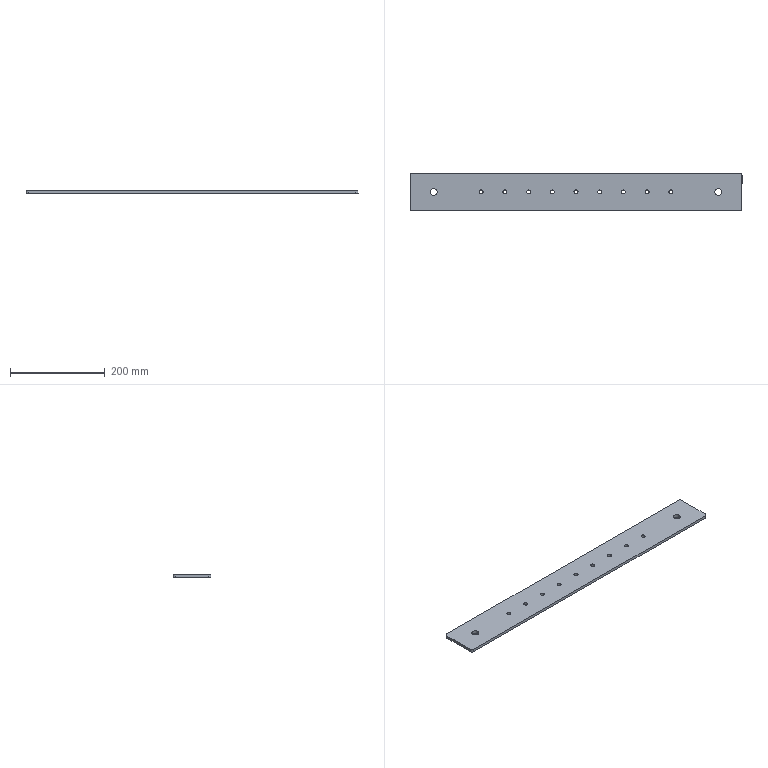Part | STEP file | 750038460 | 1 solid | 32 faces | box 700 x 80 x 6 mm | volume 330686 mm3 | cylinder 26 | plane 6 | commonest cylinder face diameters 8.5 x18 10 x4 15 x4
STEP:
#1=CARTESIAN_POINT('',(-607.5,0.,0.));
#2=VERTEX_POINT('',#1);
#3=CARTESIAN_POINT('',(-592.5,0.,0.));
#4=VERTEX_POINT('',#3);
#5=CARTESIAN_POINT('',(-600.,0.,0.));
#6=DIRECTION('',(0.,0.,1.));
#7=DIRECTION('',(1.,0.,0.));
#8=AXIS2_PLACEMENT_3D('',#5,#6,#7);
#9=CIRCLE('',#8,7.5);
#10=EDGE_CURVE('',#2,#4,#9,.T.);
#11=ORIENTED_EDGE('',*,*,#10,.F.);
#12=CARTESIAN_POINT('',(-607.5,0.,6.));
#13=VERTEX_POINT('',#12);
#14=CARTESIAN_POINT('',(-607.5,0.,-54994.));
#15=DIRECTION('',(0.,0.,1.));
#16=VECTOR('',#15,1000.);
#17=LINE('',#14,#16);
#18=EDGE_CURVE('',#2,#13,#17,.T.);
#19=ORIENTED_EDGE('',*,*,#18,.T.);
#20=CARTESIAN_POINT('',(-592.5,0.,6.));
#21=VERTEX_POINT('',#20);
#22=CARTESIAN_POINT('',(-600.,0.,6.));
#23=DIRECTION('',(0.,0.,-1.));
#24=DIRECTION('',(1.,0.,0.));
#25=AXIS2_PLACEMENT_3D('',#22,#23,#24);
#26=CIRCLE('',#25,7.5);
#27=EDGE_CURVE('',#21,#13,#26,.T.);
#28=ORIENTED_EDGE('',*,*,#27,.F.);
#29=CARTESIAN_POINT('',(-592.5,0.,-54994.));
#30=DIRECTION('',(0.,0.,1.));
#31=VECTOR('',#30,1000.);
#32=LINE('',#29,#31);
#33=EDGE_CURVE('',#4,#21,#32,.T.);
#34=ORIENTED_EDGE('',*,*,#33,.F.);
#35=EDGE_LOOP('',(#11,#19,#28,#34));
#36=FACE_OUTER_BOUND('',#35,.T.);
#37=CARTESIAN_POINT('',(-600.,0.,-54994.));
#38=DIRECTION('',(0.,0.,1.));
#39=DIRECTION('',(1.,0.,0.));
#40=AXIS2_PLACEMENT_3D('',#37,#38,#39);
#41=CYLINDRICAL_SURFACE('',#40,7.5);
#42=ADVANCED_FACE('',(#36),#41,.F.);
#43=CARTESIAN_POINT('',(-504.25,0.,0.));
#44=VERTEX_POINT('',#43);
#45=CARTESIAN_POINT('',(-495.75,0.,0.));
#46=VERTEX_POINT('',#45);
#47=CARTESIAN_POINT('',(-500.,0.,0.));
#48=DIRECTION('',(0.,0.,1.));
#49=DIRECTION('',(1.,0.,0.));
#50=AXIS2_PLACEMENT_3D('',#47,#48,#49);
#51=CIRCLE('',#50,4.25);
#52=EDGE_CURVE('',#44,#46,#51,.T.);
#53=ORIENTED_EDGE('',*,*,#52,.F.);
#54=CARTESIAN_POINT('',(-504.25,0.,6.));
#55=VERTEX_POINT('',#54);
#56=CARTESIAN_POINT('',(-504.25,0.,-54994.));
#57=DIRECTION('',(0.,0.,1.));
#58=VECTOR('',#57,1000.);
#59=LINE('',#56,#58);
#60=EDGE_CURVE('',#44,#55,#59,.T.);
#61=ORIENTED_EDGE('',*,*,#60,.T.);
#62=CARTESIAN_POINT('',(-495.75,0.,6.));
#63=VERTEX_POINT('',#62);
#64=CARTESIAN_POINT('',(-500.,0.,6.));
#65=DIRECTION('',(0.,0.,-1.));
#66=DIRECTION('',(1.,0.,0.));
#67=AXIS2_PLACEMENT_3D('',#64,#65,#66);
#68=CIRCLE('',#67,4.25);
#69=EDGE_CURVE('',#63,#55,#68,.T.);
#70=ORIENTED_EDGE('',*,*,#69,.F.);
#71=CARTESIAN_POINT('',(-495.75,0.,-54994.));
#72=DIRECTION('',(0.,0.,1.));
#73=VECTOR('',#72,1000.);
#74=LINE('',#71,#73);
#75=EDGE_CURVE('',#46,#63,#74,.T.);
#76=ORIENTED_EDGE('',*,*,#75,.F.);
#77=EDGE_LOOP('',(#53,#61,#70,#76));
#78=FACE_OUTER_BOUND('',#77,.T.);
#79=CARTESIAN_POINT('',(-500.,0.,-54994.));
#80=DIRECTION('',(0.,0.,1.));
#81=DIRECTION('',(1.,0.,0.));
#82=AXIS2_PLACEMENT_3D('',#79,#80,#81);
#83=CYLINDRICAL_SURFACE('',#82,4.25);
#84=ADVANCED_FACE('',(#78),#83,.F.);
#85=CARTESIAN_POINT('',(-454.25,0.,0.));
#86=VERTEX_POINT('',#85);
#87=CARTESIAN_POINT('',(-445.75,0.,0.));
#88=VERTEX_POINT('',#87);
#89=CARTESIAN_POINT('',(-450.,0.,0.));
#90=DIRECTION('',(0.,0.,1.));
#91=DIRECTION('',(1.,0.,0.));
#92=AXIS2_PLACEMENT_3D('',#89,#90,#91);
#93=CIRCLE('',#92,4.25);
#94=EDGE_CURVE('',#86,#88,#93,.T.);
#95=ORIENTED_EDGE('',*,*,#94,.F.);
#96=CARTESIAN_POINT('',(-454.25,0.,6.));
#97=VERTEX_POINT('',#96);
#98=CARTESIAN_POINT('',(-454.25,0.,-54994.));
#99=DIRECTION('',(0.,0.,1.));
#100=VECTOR('',#99,1000.);
#101=LINE('',#98,#100);
#102=EDGE_CURVE('',#86,#97,#101,.T.);
#103=ORIENTED_EDGE('',*,*,#102,.T.);
#104=CARTESIAN_POINT('',(-445.75,0.,6.));
#105=VERTEX_POINT('',#104);
#106=CARTESIAN_POINT('',(-450.,0.,6.));
#107=DIRECTION('',(0.,0.,-1.));
#108=DIRECTION('',(1.,0.,0.));
#109=AXIS2_PLACEMENT_3D('',#106,#107,#108);
#110=CIRCLE('',#109,4.25);
#111=EDGE_CURVE('',#105,#97,#110,.T.);
#112=ORIENTED_EDGE('',*,*,#111,.F.);
#113=CARTESIAN_POINT('',(-445.75,0.,-54994.));
#114=DIRECTION('',(0.,0.,1.));
#115=VECTOR('',#114,1000.);
#116=LINE('',#113,#115);
#117=EDGE_CURVE('',#88,#105,#116,.T.);
#118=ORIENTED_EDGE('',*,*,#117,.F.);
#119=EDGE_LOOP('',(#95,#103,#112,#118));
#120=FACE_OUTER_BOUND('',#119,.T.);
#121=CARTESIAN_POINT('',(-450.,0.,-54994.));
#122=DIRECTION('',(0.,0.,1.));
#123=DIRECTION('',(1.,0.,0.));
#124=AXIS2_PLACEMENT_3D('',#121,#122,#123);
#125=CYLINDRICAL_SURFACE('',#124,4.25);
#126=ADVANCED_FACE('',(#120),#125,.F.);
#127=CARTESIAN_POINT('',(-404.25,0.,0.));
#128=VERTEX_POINT('',#127);
#129=CARTESIAN_POINT('',(-395.75,0.,0.));
#130=VERTEX_POINT('',#129);
#131=CARTESIAN_POINT('',(-400.,0.,0.));
#132=DIRECTION('',(0.,0.,1.));
#133=DIRECTION('',(1.,0.,0.));
#134=AXIS2_PLACEMENT_3D('',#131,#132,#133);
#135=CIRCLE('',#134,4.25);
#136=EDGE_CURVE('',#128,#130,#135,.T.);
#137=ORIENTED_EDGE('',*,*,#136,.F.);
#138=CARTESIAN_POINT('',(-404.25,0.,6.));
#139=VERTEX_POINT('',#138);
#140=CARTESIAN_POINT('',(-404.25,0.,-54994.));
#141=DIRECTION('',(0.,0.,1.));
#142=VECTOR('',#141,1000.);
#143=LINE('',#140,#142);
#144=EDGE_CURVE('',#128,#139,#143,.T.);
#145=ORIENTED_EDGE('',*,*,#144,.T.);
#146=CARTESIAN_POINT('',(-395.75,0.,6.));
#147=VERTEX_POINT('',#146);
#148=CARTESIAN_POINT('',(-400.,0.,6.));
#149=DIRECTION('',(0.,0.,-1.));
#150=DIRECTION('',(1.,0.,0.));
#151=AXIS2_PLACEMENT_3D('',#148,#149,#150);
#152=CIRCLE('',#151,4.25);
#153=EDGE_CURVE('',#147,#139,#152,.T.);
#154=ORIENTED_EDGE('',*,*,#153,.F.);
#155=CARTESIAN_POINT('',(-395.75,0.,-54994.));
#156=DIRECTION('',(0.,0.,1.));
#157=VECTOR('',#156,1000.);
#158=LINE('',#155,#157);
#159=EDGE_CURVE('',#130,#147,#158,.T.);
#160=ORIENTED_EDGE('',*,*,#159,.F.);
#161=EDGE_LOOP('',(#137,#145,#154,#160));
#162=FACE_OUTER_BOUND('',#161,.T.);
#163=CARTESIAN_POINT('',(-400.,0.,-54994.));
#164=DIRECTION('',(0.,0.,1.));
#165=DIRECTION('',(1.,0.,0.));
#166=AXIS2_PLACEMENT_3D('',#163,#164,#165);
#167=CYLINDRICAL_SURFACE('',#166,4.25);
#168=ADVANCED_FACE('',(#162),#167,.F.);
#169=CARTESIAN_POINT('',(-354.25,0.,0.));
#170=VERTEX_POINT('',#169);
#171=CARTESIAN_POINT('',(-345.75,0.,0.));
#172=VERTEX_POINT('',#171);
#173=CARTESIAN_POINT('',(-350.,0.,0.));
#174=DIRECTION('',(0.,0.,1.));
#175=DIRECTION('',(1.,0.,0.));
#176=AXIS2_PLACEMENT_3D('',#173,#174,#175);
#177=CIRCLE('',#176,4.25);
#178=EDGE_CURVE('',#170,#172,#177,.T.);
#179=ORIENTED_EDGE('',*,*,#178,.F.);
#180=CARTESIAN_POINT('',(-354.25,0.,6.));
#181=VERTEX_POINT('',#180);
#182=CARTESIAN_POINT('',(-354.25,0.,-54994.));
#183=DIRECTION('',(0.,0.,1.));
#184=VECTOR('',#183,1000.);
#185=LINE('',#182,#184);
#186=EDGE_CURVE('',#170,#181,#185,.T.);
#187=ORIENTED_EDGE('',*,*,#186,.T.);
#188=CARTESIAN_POINT('',(-345.75,0.,6.));
#189=VERTEX_POINT('',#188);
#190=CARTESIAN_POINT('',(-350.,0.,6.));
#191=DIRECTION('',(0.,0.,-1.));
#192=DIRECTION('',(1.,0.,0.));
#193=AXIS2_PLACEMENT_3D('',#190,#191,#192);
#194=CIRCLE('',#193,4.25);
#195=EDGE_CURVE('',#189,#181,#194,.T.);
#196=ORIENTED_EDGE('',*,*,#195,.F.);
#197=CARTESIAN_POINT('',(-345.75,0.,-54994.));
#198=DIRECTION('',(0.,0.,1.));
#199=VECTOR('',#198,1000.);
#200=LINE('',#197,#199);
#201=EDGE_CURVE('',#172,#189,#200,.T.);
#202=ORIENTED_EDGE('',*,*,#201,.F.);
#203=EDGE_LOOP('',(#179,#187,#196,#202));
#204=FACE_OUTER_BOUND('',#203,.T.);
#205=CARTESIAN_POINT('',(-350.,0.,-54994.));
#206=DIRECTION('',(0.,0.,1.));
#207=DIRECTION('',(1.,0.,0.));
#208=AXIS2_PLACEMENT_3D('',#205,#206,#207);
#209=CYLINDRICAL_SURFACE('',#208,4.25);
#210=ADVANCED_FACE('',(#204),#209,.F.);
#211=CARTESIAN_POINT('',(-304.25,0.,0.));
#212=VERTEX_POINT('',#211);
#213=CARTESIAN_POINT('',(-295.75,0.,0.));
#214=VERTEX_POINT('',#213);
#215=CARTESIAN_POINT('',(-300.,0.,0.));
#216=DIRECTION('',(0.,0.,1.));
#217=DIRECTION('',(1.,0.,0.));
#218=AXIS2_PLACEMENT_3D('',#215,#216,#217);
#219=CIRCLE('',#218,4.25);
#220=EDGE_CURVE('',#212,#214,#219,.T.);
#221=ORIENTED_EDGE('',*,*,#220,.F.);
#222=CARTESIAN_POINT('',(-304.25,0.,6.));
#223=VERTEX_POINT('',#222);
#224=CARTESIAN_POINT('',(-304.25,0.,-54994.));
#225=DIRECTION('',(0.,0.,1.));
#226=VECTOR('',#225,1000.);
#227=LINE('',#224,#226);
#228=EDGE_CURVE('',#212,#223,#227,.T.);
#229=ORIENTED_EDGE('',*,*,#228,.T.);
#230=CARTESIAN_POINT('',(-295.75,0.,6.));
#231=VERTEX_POINT('',#230);
#232=CARTESIAN_POINT('',(-300.,0.,6.));
#233=DIRECTION('',(0.,0.,-1.));
#234=DIRECTION('',(1.,0.,0.));
#235=AXIS2_PLACEMENT_3D('',#232,#233,#234);
#236=CIRCLE('',#235,4.25);
#237=EDGE_CURVE('',#231,#223,#236,.T.);
#238=ORIENTED_EDGE('',*,*,#237,.F.);
#239=CARTESIAN_POINT('',(-295.75,0.,-54994.));
#240=DIRECTION('',(0.,0.,1.));
#241=VECTOR('',#240,1000.);
#242=LINE('',#239,#241);
#243=EDGE_CURVE('',#214,#231,#242,.T.);
#244=ORIENTED_EDGE('',*,*,#243,.F.);
#245=EDGE_LOOP('',(#221,#229,#238,#244));
#246=FACE_OUTER_BOUND('',#245,.T.);
#247=CARTESIAN_POINT('',(-300.,0.,-54994.));
#248=DIRECTION('',(0.,0.,1.));
#249=DIRECTION('',(1.,0.,0.));
#250=AXIS2_PLACEMENT_3D('',#247,#248,#249);
#251=CYLINDRICAL_SURFACE('',#250,4.25);
#252=ADVANCED_FACE('',(#246),#251,.F.);
#253=CARTESIAN_POINT('',(-254.25,0.,0.));
#254=VERTEX_POINT('',#253);
#255=CARTESIAN_POINT('',(-245.75,0.,0.));
#256=VERTEX_POINT('',#255);
#257=CARTESIAN_POINT('',(-250.,0.,0.));
#258=DIRECTION('',(0.,0.,1.));
#259=DIRECTION('',(1.,0.,0.));
#260=AXIS2_PLACEMENT_3D('',#257,#258,#259);
#261=CIRCLE('',#260,4.25);
#262=EDGE_CURVE('',#254,#256,#261,.T.);
#263=ORIENTED_EDGE('',*,*,#262,.F.);
#264=CARTESIAN_POINT('',(-254.25,0.,6.));
#265=VERTEX_POINT('',#264);
#266=CARTESIAN_POINT('',(-254.25,0.,-54994.));
#267=DIRECTION('',(0.,0.,1.));
#268=VECTOR('',#267,1000.);
#269=LINE('',#266,#268);
#270=EDGE_CURVE('',#254,#265,#269,.T.);
#271=ORIENTED_EDGE('',*,*,#270,.T.);
#272=CARTESIAN_POINT('',(-245.75,0.,6.));
#273=VERTEX_POINT('',#272);
#274=CARTESIAN_POINT('',(-250.,0.,6.));
#275=DIRECTION('',(0.,0.,-1.));
#276=DIRECTION('',(1.,0.,0.));
#277=AXIS2_PLACEMENT_3D('',#274,#275,#276);
#278=CIRCLE('',#277,4.25);
#279=EDGE_CURVE('',#273,#265,#278,.T.);
#280=ORIENTED_EDGE('',*,*,#279,.F.);
#281=CARTESIAN_POINT('',(-245.75,0.,-54994.));
#282=DIRECTION('',(0.,0.,1.));
#283=VECTOR('',#282,1000.);
#284=LINE('',#281,#283);
#285=EDGE_CURVE('',#256,#273,#284,.T.);
#286=ORIENTED_EDGE('',*,*,#285,.F.);
#287=EDGE_LOOP('',(#263,#271,#280,#286));
#288=FACE_OUTER_BOUND('',#287,.T.);
#289=CARTESIAN_POINT('',(-250.,0.,-54994.));
#290=DIRECTION('',(0.,0.,1.));
#291=DIRECTION('',(1.,0.,0.));
#292=AXIS2_PLACEMENT_3D('',#289,#290,#291);
#293=CYLINDRICAL_SURFACE('',#292,4.25);
#294=ADVANCED_FACE('',(#288),#293,.F.);
#295=CARTESIAN_POINT('',(-204.25,0.,0.));
#296=VERTEX_POINT('',#295);
#297=CARTESIAN_POINT('',(-195.75,0.,0.));
#298=VERTEX_POINT('',#297);
#299=CARTESIAN_POINT('',(-200.,0.,0.));
#300=DIRECTION('',(0.,0.,1.));
#301=DIRECTION('',(1.,0.,0.));
#302=AXIS2_PLACEMENT_3D('',#299,#300,#301);
#303=CIRCLE('',#302,4.25);
#304=EDGE_CURVE('',#296,#298,#303,.T.);
#305=ORIENTED_EDGE('',*,*,#304,.F.);
#306=CARTESIAN_POINT('',(-204.25,0.,6.));
#307=VERTEX_POINT('',#306);
#308=CARTESIAN_POINT('',(-204.25,0.,-54994.));
#309=DIRECTION('',(0.,0.,1.));
#310=VECTOR('',#309,1000.);
#311=LINE('',#308,#310);
#312=EDGE_CURVE('',#296,#307,#311,.T.);
#313=ORIENTED_EDGE('',*,*,#312,.T.);
#314=CARTESIAN_POINT('',(-195.75,0.,6.));
#315=VERTEX_POINT('',#314);
#316=CARTESIAN_POINT('',(-200.,0.,6.));
#317=DIRECTION('',(0.,0.,-1.));
#318=DIRECTION('',(1.,0.,0.));
#319=AXIS2_PLACEMENT_3D('',#316,#317,#318);
#320=CIRCLE('',#319,4.25);
#321=EDGE_CURVE('',#315,#307,#320,.T.);
#322=ORIENTED_EDGE('',*,*,#321,.F.);
#323=CARTESIAN_POINT('',(-195.75,0.,-54994.));
#324=DIRECTION('',(0.,0.,1.));
#325=VECTOR('',#324,1000.);
#326=LINE('',#323,#325);
#327=EDGE_CURVE('',#298,#315,#326,.T.);
#328=ORIENTED_EDGE('',*,*,#327,.F.);
#329=EDGE_LOOP('',(#305,#313,#322,#328));
#330=FACE_OUTER_BOUND('',#329,.T.);
#331=CARTESIAN_POINT('',(-200.,0.,-54994.));
#332=DIRECTION('',(0.,0.,1.));
#333=DIRECTION('',(1.,0.,0.));
#334=AXIS2_PLACEMENT_3D('',#331,#332,#333);
#335=CYLINDRICAL_SURFACE('',#334,4.25);
#336=ADVANCED_FACE('',(#330),#335,.F.);
#337=CARTESIAN_POINT('',(-154.25,0.,0.));
#338=VERTEX_POINT('',#337);
#339=CARTESIAN_POINT('',(-145.75,0.,0.));
#340=VERTEX_POINT('',#339);
#341=CARTESIAN_POINT('',(-150.,0.,0.));
#342=DIRECTION('',(0.,0.,1.));
#343=DIRECTION('',(1.,0.,0.));
#344=AXIS2_PLACEMENT_3D('',#341,#342,#343);
#345=CIRCLE('',#344,4.25);
#346=EDGE_CURVE('',#338,#340,#345,.T.);
#347=ORIENTED_EDGE('',*,*,#346,.F.);
#348=CARTESIAN_POINT('',(-154.25,0.,6.));
#349=VERTEX_POINT('',#348);
#350=CARTESIAN_POINT('',(-154.25,0.,-54994.));
#351=DIRECTION('',(0.,0.,1.));
#352=VECTOR('',#351,1000.);
#353=LINE('',#350,#352);
#354=EDGE_CURVE('',#338,#349,#353,.T.);
#355=ORIENTED_EDGE('',*,*,#354,.T.);
#356=CARTESIAN_POINT('',(-145.75,0.,6.));
#357=VERTEX_POINT('',#356);
#358=CARTESIAN_POINT('',(-150.,0.,6.));
#359=DIRECTION('',(0.,0.,-1.));
#360=DIRECTION('',(1.,0.,0.));
#361=AXIS2_PLACEMENT_3D('',#358,#359,#360);
#362=CIRCLE('',#361,4.25);
#363=EDGE_CURVE('',#357,#349,#362,.T.);
#364=ORIENTED_EDGE('',*,*,#363,.F.);
#365=CARTESIAN_POINT('',(-145.75,0.,-54994.));
#366=DIRECTION('',(0.,0.,1.));
#367=VECTOR('',#366,1000.);
#368=LINE('',#365,#367);
#369=EDGE_CURVE('',#340,#357,#368,.T.);
#370=ORIENTED_EDGE('',*,*,#369,.F.);
#371=EDGE_LOOP('',(#347,#355,#364,#370));
#372=FACE_OUTER_BOUND('',#371,.T.);
#373=CARTESIAN_POINT('',(-150.,0.,-54994.));
#374=DIRECTION('',(0.,0.,1.));
#375=DIRECTION('',(1.,0.,0.));
#376=AXIS2_PLACEMENT_3D('',#373,#374,#375);
#377=CYLINDRICAL_SURFACE('',#376,4.25);
#378=ADVANCED_FACE('',(#372),#377,.F.);
#379=CARTESIAN_POINT('',(-104.25,0.,0.));
#380=VERTEX_POINT('',#379);
#381=CARTESIAN_POINT('',(-95.75,0.,0.));
#382=VERTEX_POINT('',#381);
#383=CARTESIAN_POINT('',(-100.,0.,0.));
#384=DIRECTION('',(0.,0.,1.));
#385=DIRECTION('',(1.,0.,0.));
#386=AXIS2_PLACEMENT_3D('',#383,#384,#385);
#387=CIRCLE('',#386,4.25);
#388=EDGE_CURVE('',#380,#382,#387,.T.);
#389=ORIENTED_EDGE('',*,*,#388,.F.);
#390=CARTESIAN_POINT('',(-104.25,0.,6.));
#391=VERTEX_POINT('',#390);
#392=CARTESIAN_POINT('',(-104.25,0.,-54994.));
#393=DIRECTION('',(0.,0.,1.));
#394=VECTOR('',#393,1000.);
#395=LINE('',#392,#394);
#396=EDGE_CURVE('',#380,#391,#395,.T.);
#397=ORIENTED_EDGE('',*,*,#396,.T.);
#398=CARTESIAN_POINT('',(-95.75,0.,6.));
#399=VERTEX_POINT('',#398);
#400=CARTESIAN_POINT('',(-100.,0.,6.));
#401=DIRECTION('',(0.,0.,-1.));
#402=DIRECTION('',(1.,0.,0.));
#403=AXIS2_PLACEMENT_3D('',#400,#401,#402);
#404=CIRCLE('',#403,4.25);
#405=EDGE_CURVE('',#399,#391,#404,.T.);
#406=ORIENTED_EDGE('',*,*,#405,.F.);
#407=CARTESIAN_POINT('',(-95.75,0.,-54994.));
#408=DIRECTION('',(0.,0.,1.));
#409=VECTOR('',#408,1000.);
#410=LINE('',#407,#409);
#411=EDGE_CURVE('',#382,#399,#410,.T.);
#412=ORIENTED_EDGE('',*,*,#411,.F.);
#413=EDGE_LOOP('',(#389,#397,#406,#412));
#414=FACE_OUTER_BOUND('',#413,.T.);
#415=CARTESIAN_POINT('',(-100.,0.,-54994.));
#416=DIRECTION('',(0.,0.,1.));
#417=DIRECTION('',(1.,0.,0.));
#418=AXIS2_PLACEMENT_3D('',#415,#416,#417);
#419=CYLINDRICAL_SURFACE('',#418,4.25);
#420=ADVANCED_FACE('',(#414),#419,.F.);
#421=CARTESIAN_POINT('',(-7.5,0.,0.));
#422=VERTEX_POINT('',#421);
#423=CARTESIAN_POINT('',(7.5,0.,0.));
#424=VERTEX_POINT('',#423);
#425=CARTESIAN_POINT('',(0.,0.,0.));
#426=DIRECTION('',(0.,0.,1.));
#427=DIRECTION('',(1.,0.,0.));
#428=AXIS2_PLACEMENT_3D('',#425,#426,#427);
#429=CIRCLE('',#428,7.5);
#430=EDGE_CURVE('',#422,#424,#429,.T.);
#431=ORIENTED_EDGE('',*,*,#430,.F.);
#432=CARTESIAN_POINT('',(-7.5,0.,6.));
#433=VERTEX_POINT('',#432);
#434=CARTESIAN_POINT('',(-7.5,0.,-54994.));
#435=DIRECTION('',(0.,0.,1.));
#436=VECTOR('',#435,1000.);
#437=LINE('',#434,#436);
#438=EDGE_CURVE('',#422,#433,#437,.T.);
#439=ORIENTED_EDGE('',*,*,#438,.T.);
#440=CARTESIAN_POINT('',(7.5,0.,6.));
#441=VERTEX_POINT('',#440);
#442=CARTESIAN_POINT('',(0.,0.,6.));
#443=DIRECTION('',(0.,0.,-1.));
#444=DIRECTION('',(1.,0.,0.));
#445=AXIS2_PLACEMENT_3D('',#442,#443,#444);
#446=CIRCLE('',#445,7.5);
#447=EDGE_CURVE('',#441,#433,#446,.T.);
#448=ORIENTED_EDGE('',*,*,#447,.F.);
#449=CARTESIAN_POINT('',(7.5,0.,-54994.));
#450=DIRECTION('',(0.,0.,1.));
#451=VECTOR('',#450,1000.);
#452=LINE('',#449,#451);
#453=EDGE_CURVE('',#424,#441,#452,.T.);
#454=ORIENTED_EDGE('',*,*,#453,.F.);
#455=EDGE_LOOP('',(#431,#439,#448,#454));
#456=FACE_OUTER_BOUND('',#455,.T.);
#457=CARTESIAN_POINT('',(0.,0.,-54994.));
#458=DIRECTION('',(0.,0.,1.));
#459=DIRECTION('',(1.,0.,0.));
#460=AXIS2_PLACEMENT_3D('',#457,#458,#459);
#461=CYLINDRICAL_SURFACE('',#460,7.5);
#462=ADVANCED_FACE('',(#456),#461,.F.);
#463=CARTESIAN_POINT('',(45.,40.,6.));
#464=VERTEX_POINT('',#463);
#465=CARTESIAN_POINT('',(-645.,40.,6.));
#466=VERTEX_POINT('',#465);
#467=CARTESIAN_POINT('',(-645.,40.,6.));
#468=DIRECTION('',(-1.,0.,0.));
#469=VECTOR('',#468,1000.);
#470=LINE('',#467,#469);
#471=EDGE_CURVE('',#464,#466,#470,.T.);
#472=ORIENTED_EDGE('',*,*,#471,.T.);
#473=CARTESIAN_POINT('',(-650.,35.,6.));
#474=VERTEX_POINT('',#473);
#475=CARTESIAN_POINT('',(-645.,35.,6.));
#476=DIRECTION('',(0.,0.,1.));
#477=DIRECTION('',(-1.,0.,0.));
#478=AXIS2_PLACEMENT_3D('',#475,#476,#477);
#479=CIRCLE('',#478,5.);
#480=EDGE_CURVE('',#466,#474,#479,.T.);
#481=ORIENTED_EDGE('',*,*,#480,.T.);
#482=CARTESIAN_POINT('',(-650.,-35.,6.));
#483=VERTEX_POINT('',#482);
#484=CARTESIAN_POINT('',(-650.,-35.,6.));
#485=DIRECTION('',(0.,-1.,0.));
#486=VECTOR('',#485,1000.);
#487=LINE('',#484,#486);
#488=EDGE_CURVE('',#474,#483,#487,.T.);
#489=ORIENTED_EDGE('',*,*,#488,.T.);
#490=CARTESIAN_POINT('',(-645.,-40.,6.));
#491=VERTEX_POINT('',#490);
#492=CARTESIAN_POINT('',(-645.,-35.,6.));
#493=DIRECTION('',(0.,0.,1.));
#494=DIRECTION('',(-1.,0.,0.));
#495=AXIS2_PLACEMENT_3D('',#492,#493,#494);
#496=CIRCLE('',#495,5.);
#497=EDGE_CURVE('',#483,#491,#496,.T.);
#498=ORIENTED_EDGE('',*,*,#497,.T.);
#499=CARTESIAN_POINT('',(45.,-40.,6.));
#500=VERTEX_POINT('',#499);
#501=CARTESIAN_POINT('',(-645.,-40.,6.));
#502=DIRECTION('',(1.,0.,0.));
#503=VECTOR('',#502,1000.);
#504=LINE('',#501,#503);
#505=EDGE_CURVE('',#491,#500,#504,.T.);
#506=ORIENTED_EDGE('',*,*,#505,.T.);
#507=CARTESIAN_POINT('',(50.,-35.,6.));
#508=VERTEX_POINT('',#507);
#509=CARTESIAN_POINT('',(45.,-35.,6.));
#510=DIRECTION('',(0.,0.,1.));
#511=DIRECTION('',(-1.,0.,0.));
#512=AXIS2_PLACEMENT_3D('',#509,#510,#511);
#513=CIRCLE('',#512,5.);
#514=EDGE_CURVE('',#500,#508,#513,.T.);
#515=ORIENTED_EDGE('',*,*,#514,.T.);
#516=CARTESIAN_POINT('',(50.,35.,6.));
#517=VERTEX_POINT('',#516);
#518=CARTESIAN_POINT('',(50.,-35.,6.));
#519=DIRECTION('',(0.,1.,0.));
#520=VECTOR('',#519,1000.);
#521=LINE('',#518,#520);
#522=EDGE_CURVE('',#508,#517,#521,.T.);
#523=ORIENTED_EDGE('',*,*,#522,.T.);
#524=CARTESIAN_POINT('',(45.,35.,6.));
#525=DIRECTION('',(0.,0.,1.));
#526=DIRECTION('',(-1.,0.,0.));
#527=AXIS2_PLACEMENT_3D('',#524,#525,#526);
#528=CIRCLE('',#527,5.);
#529=EDGE_CURVE('',#517,#464,#528,.T.);
#530=ORIENTED_EDGE('',*,*,#529,.T.);
#531=EDGE_LOOP('',(#472,#481,#489,#498,#506,#515,#523,#530));
#532=FACE_OUTER_BOUND('',#531,.T.);
#533=ORIENTED_EDGE('',*,*,#27,.T.);
#534=CARTESIAN_POINT('',(-600.,0.,6.));
#535=DIRECTION('',(0.,0.,-1.));
#536=DIRECTION('',(1.,0.,0.));
#537=AXIS2_PLACEMENT_3D('',#534,#535,#536);
#538=CIRCLE('',#537,7.5);
#539=EDGE_CURVE('',#13,#21,#538,.T.);
#540=ORIENTED_EDGE('',*,*,#539,.T.);
#541=EDGE_LOOP('',(#533,#540));
#542=FACE_BOUND('',#541,.T.);
#543=ORIENTED_EDGE('',*,*,#69,.T.);
#544=CARTESIAN_POINT('',(-500.,0.,6.));
#545=DIRECTION('',(0.,0.,-1.));
#546=DIRECTION('',(1.,0.,0.));
#547=AXIS2_PLACEMENT_3D('',#544,#545,#546);
#548=CIRCLE('',#547,4.25);
#549=EDGE_CURVE('',#55,#63,#548,.T.);
#550=ORIENTED_EDGE('',*,*,#549,.T.);
#551=EDGE_LOOP('',(#543,#550));
#552=FACE_BOUND('',#551,.T.);
#553=ORIENTED_EDGE('',*,*,#111,.T.);
#554=CARTESIAN_POINT('',(-450.,0.,6.));
#555=DIRECTION('',(0.,0.,-1.));
#556=DIRECTION('',(1.,0.,0.));
#557=AXIS2_PLACEMENT_3D('',#554,#555,#556);
#558=CIRCLE('',#557,4.25);
#559=EDGE_CURVE('',#97,#105,#558,.T.);
#560=ORIENTED_EDGE('',*,*,#559,.T.);
#561=EDGE_LOOP('',(#553,#560));
#562=FACE_BOUND('',#561,.T.);
#563=ORIENTED_EDGE('',*,*,#153,.T.);
#564=CARTESIAN_POINT('',(-400.,0.,6.));
#565=DIRECTION('',(0.,0.,-1.));
#566=DIRECTION('',(1.,0.,0.));
#567=AXIS2_PLACEMENT_3D('',#564,#565,#566);
#568=CIRCLE('',#567,4.25);
#569=EDGE_CURVE('',#139,#147,#568,.T.);
#570=ORIENTED_EDGE('',*,*,#569,.T.);
#571=EDGE_LOOP('',(#563,#570));
#572=FACE_BOUND('',#571,.T.);
#573=ORIENTED_EDGE('',*,*,#195,.T.);
#574=CARTESIAN_POINT('',(-350.,0.,6.));
#575=DIRECTION('',(0.,0.,-1.));
#576=DIRECTION('',(1.,0.,0.));
#577=AXIS2_PLACEMENT_3D('',#574,#575,#576);
#578=CIRCLE('',#577,4.25);
#579=EDGE_CURVE('',#181,#189,#578,.T.);
#580=ORIENTED_EDGE('',*,*,#579,.T.);
#581=EDGE_LOOP('',(#573,#580));
#582=FACE_BOUND('',#581,.T.);
#583=ORIENTED_EDGE('',*,*,#237,.T.);
#584=CARTESIAN_POINT('',(-300.,0.,6.));
#585=DIRECTION('',(0.,0.,-1.));
#586=DIRECTION('',(1.,0.,0.));
#587=AXIS2_PLACEMENT_3D('',#584,#585,#586);
#588=CIRCLE('',#587,4.25);
#589=EDGE_CURVE('',#223,#231,#588,.T.);
#590=ORIENTED_EDGE('',*,*,#589,.T.);
#591=EDGE_LOOP('',(#583,#590));
#592=FACE_BOUND('',#591,.T.);
#593=ORIENTED_EDGE('',*,*,#279,.T.);
#594=CARTESIAN_POINT('',(-250.,0.,6.));
#595=DIRECTION('',(0.,0.,-1.));
#596=DIRECTION('',(1.,0.,0.));
#597=AXIS2_PLACEMENT_3D('',#594,#595,#596);
#598=CIRCLE('',#597,4.25);
#599=EDGE_CURVE('',#265,#273,#598,.T.);
#600=ORIENTED_EDGE('',*,*,#599,.T.);
#601=EDGE_LOOP('',(#593,#600));
#602=FACE_BOUND('',#601,.T.);
#603=ORIENTED_EDGE('',*,*,#321,.T.);
#604=CARTESIAN_POINT('',(-200.,0.,6.));
#605=DIRECTION('',(0.,0.,-1.));
#606=DIRECTION('',(1.,0.,0.));
#607=AXIS2_PLACEMENT_3D('',#604,#605,#606);
#608=CIRCLE('',#607,4.25);
#609=EDGE_CURVE('',#307,#315,#608,.T.);
#610=ORIENTED_EDGE('',*,*,#609,.T.);
#611=EDGE_LOOP('',(#603,#610));
#612=FACE_BOUND('',#611,.T.);
#613=ORIENTED_EDGE('',*,*,#363,.T.);
#614=CARTESIAN_POINT('',(-150.,0.,6.));
#615=DIRECTION('',(0.,0.,-1.));
#616=DIRECTION('',(1.,0.,0.));
#617=AXIS2_PLACEMENT_3D('',#614,#615,#616);
#618=CIRCLE('',#617,4.25);
#619=EDGE_CURVE('',#349,#357,#618,.T.);
#620=ORIENTED_EDGE('',*,*,#619,.T.);
#621=EDGE_LOOP('',(#613,#620));
#622=FACE_BOUND('',#621,.T.);
#623=ORIENTED_EDGE('',*,*,#405,.T.);
#624=CARTESIAN_POINT('',(-100.,0.,6.));
#625=DIRECTION('',(0.,0.,-1.));
#626=DIRECTION('',(1.,0.,0.));
#627=AXIS2_PLACEMENT_3D('',#624,#625,#626);
#628=CIRCLE('',#627,4.25);
#629=EDGE_CURVE('',#391,#399,#628,.T.);
#630=ORIENTED_EDGE('',*,*,#629,.T.);
#631=EDGE_LOOP('',(#623,#630));
#632=FACE_BOUND('',#631,.T.);
#633=ORIENTED_EDGE('',*,*,#447,.T.);
#634=CARTESIAN_POINT('',(0.,0.,6.));
#635=DIRECTION('',(0.,0.,-1.));
#636=DIRECTION('',(1.,0.,0.));
#637=AXIS2_PLACEMENT_3D('',#634,#635,#636);
#638=CIRCLE('',#637,7.5);
#639=EDGE_CURVE('',#433,#441,#638,.T.);
#640=ORIENTED_EDGE('',*,*,#639,.T.);
#641=EDGE_LOOP('',(#633,#640));
#642=FACE_BOUND('',#641,.T.);
#643=CARTESIAN_POINT('',(-645.,-35.,6.));
#644=DIRECTION('',(0.,0.,1.));
#645=DIRECTION('',(1.,0.,0.));
#646=AXIS2_PLACEMENT_3D('',#643,#644,#645);
#647=PLANE('',#646);
#648=ADVANCED_FACE('',(#532,#542,#552,#562,#572,#582,#592,#602,#612,#622,#632,#642),#647,.T.);
#649=ORIENTED_EDGE('',*,*,#480,.F.);
#650=CARTESIAN_POINT('',(-645.,40.,0.));
#651=VERTEX_POINT('',#650);
#652=CARTESIAN_POINT('',(-645.,40.,6.));
#653=DIRECTION('',(0.,0.,-1.));
#654=VECTOR('',#653,1000.);
#655=LINE('',#652,#654);
#656=EDGE_CURVE('',#466,#651,#655,.T.);
#657=ORIENTED_EDGE('',*,*,#656,.T.);
#658=CARTESIAN_POINT('',(-650.,35.,0.));
#659=VERTEX_POINT('',#658);
#660=CARTESIAN_POINT('',(-645.,35.,0.));
#661=DIRECTION('',(0.,0.,1.));
#662=DIRECTION('',(-1.,0.,0.));
#663=AXIS2_PLACEMENT_3D('',#660,#661,#662);
#664=CIRCLE('',#663,5.);
#665=EDGE_CURVE('',#651,#659,#664,.T.);
#666=ORIENTED_EDGE('',*,*,#665,.T.);
#667=CARTESIAN_POINT('',(-650.,35.,6.));
#668=DIRECTION('',(0.,0.,1.));
#669=VECTOR('',#668,1000.);
#670=LINE('',#667,#669);
#671=EDGE_CURVE('',#659,#474,#670,.T.);
#672=ORIENTED_EDGE('',*,*,#671,.T.);
#673=EDGE_LOOP('',(#649,#657,#666,#672));
#674=FACE_OUTER_BOUND('',#673,.T.);
#675=CARTESIAN_POINT('',(-645.,35.,6.));
#676=DIRECTION('',(0.,0.,-1.));
#677=DIRECTION('',(-1.,0.,0.));
#678=AXIS2_PLACEMENT_3D('',#675,#676,#677);
#679=CYLINDRICAL_SURFACE('',#678,5.);
#680=ADVANCED_FACE('',(#674),#679,.T.);
#681=ORIENTED_EDGE('',*,*,#656,.F.);
#682=ORIENTED_EDGE('',*,*,#471,.F.);
#683=CARTESIAN_POINT('',(45.,40.,0.));
#684=VERTEX_POINT('',#683);
#685=CARTESIAN_POINT('',(45.,40.,6.));
#686=DIRECTION('',(0.,0.,1.));
#687=VECTOR('',#686,1000.);
#688=LINE('',#685,#687);
#689=EDGE_CURVE('',#684,#464,#688,.T.);
#690=ORIENTED_EDGE('',*,*,#689,.F.);
#691=CARTESIAN_POINT('',(45.,40.,0.));
#692=DIRECTION('',(1.,0.,0.));
#693=VECTOR('',#692,1000.);
#694=LINE('',#691,#693);
#695=EDGE_CURVE('',#651,#684,#694,.T.);
#696=ORIENTED_EDGE('',*,*,#695,.F.);
#697=EDGE_LOOP('',(#681,#682,#690,#696));
#698=FACE_OUTER_BOUND('',#697,.T.);
#699=CARTESIAN_POINT('',(45.,40.,6.));
#700=DIRECTION('',(0.,-1.,0.));
#701=DIRECTION('',(0.,0.,-1.));
#702=AXIS2_PLACEMENT_3D('',#699,#700,#701);
#703=PLANE('',#702);
#704=ADVANCED_FACE('',(#698),#703,.F.);
#705=ORIENTED_EDGE('',*,*,#529,.F.);
#706=CARTESIAN_POINT('',(50.,35.,0.));
#707=VERTEX_POINT('',#706);
#708=CARTESIAN_POINT('',(50.,35.,6.));
#709=DIRECTION('',(0.,0.,-1.));
#710=VECTOR('',#709,1000.);
#711=LINE('',#708,#710);
#712=EDGE_CURVE('',#517,#707,#711,.T.);
#713=ORIENTED_EDGE('',*,*,#712,.T.);
#714=CARTESIAN_POINT('',(45.,35.,0.));
#715=DIRECTION('',(0.,0.,1.));
#716=DIRECTION('',(-1.,0.,0.));
#717=AXIS2_PLACEMENT_3D('',#714,#715,#716);
#718=CIRCLE('',#717,5.);
#719=EDGE_CURVE('',#707,#684,#718,.T.);
#720=ORIENTED_EDGE('',*,*,#719,.T.);
#721=ORIENTED_EDGE('',*,*,#689,.T.);
#722=EDGE_LOOP('',(#705,#713,#720,#721));
#723=FACE_OUTER_BOUND('',#722,.T.);
#724=CARTESIAN_POINT('',(45.,35.,6.));
#725=DIRECTION('',(0.,0.,-1.));
#726=DIRECTION('',(-1.,0.,0.));
#727=AXIS2_PLACEMENT_3D('',#724,#725,#726);
#728=CYLINDRICAL_SURFACE('',#727,5.);
#729=ADVANCED_FACE('',(#723),#728,.T.);
#730=ORIENTED_EDGE('',*,*,#712,.F.);
#731=ORIENTED_EDGE('',*,*,#522,.F.);
#732=CARTESIAN_POINT('',(50.,-35.,0.));
#733=VERTEX_POINT('',#732);
#734=CARTESIAN_POINT('',(50.,-35.,6.));
#735=DIRECTION('',(0.,0.,1.));
#736=VECTOR('',#735,1000.);
#737=LINE('',#734,#736);
#738=EDGE_CURVE('',#733,#508,#737,.T.);
#739=ORIENTED_EDGE('',*,*,#738,.F.);
#740=CARTESIAN_POINT('',(50.,-35.,0.));
#741=DIRECTION('',(0.,-1.,0.));
#742=VECTOR('',#741,1000.);
#743=LINE('',#740,#742);
#744=EDGE_CURVE('',#707,#733,#743,.T.);
#745=ORIENTED_EDGE('',*,*,#744,.F.);
#746=EDGE_LOOP('',(#730,#731,#739,#745));
#747=FACE_OUTER_BOUND('',#746,.T.);
#748=CARTESIAN_POINT('',(50.,-35.,6.));
#749=DIRECTION('',(-1.,0.,0.));
#750=DIRECTION('',(0.,-1.,0.));
#751=AXIS2_PLACEMENT_3D('',#748,#749,#750);
#752=PLANE('',#751);
#753=ADVANCED_FACE('',(#747),#752,.F.);
#754=ORIENTED_EDGE('',*,*,#514,.F.);
#755=CARTESIAN_POINT('',(45.,-40.,0.));
#756=VERTEX_POINT('',#755);
#757=CARTESIAN_POINT('',(45.,-40.,6.));
#758=DIRECTION('',(0.,0.,-1.));
#759=VECTOR('',#758,1000.);
#760=LINE('',#757,#759);
#761=EDGE_CURVE('',#500,#756,#760,.T.);
#762=ORIENTED_EDGE('',*,*,#761,.T.);
#763=CARTESIAN_POINT('',(45.,-35.,0.));
#764=DIRECTION('',(0.,0.,1.));
#765=DIRECTION('',(-1.,0.,0.));
#766=AXIS2_PLACEMENT_3D('',#763,#764,#765);
#767=CIRCLE('',#766,5.);
#768=EDGE_CURVE('',#756,#733,#767,.T.);
#769=ORIENTED_EDGE('',*,*,#768,.T.);
#770=ORIENTED_EDGE('',*,*,#738,.T.);
#771=EDGE_LOOP('',(#754,#762,#769,#770));
#772=FACE_OUTER_BOUND('',#771,.T.);
#773=CARTESIAN_POINT('',(45.,-35.,6.));
#774=DIRECTION('',(0.,0.,-1.));
#775=DIRECTION('',(-1.,0.,0.));
#776=AXIS2_PLACEMENT_3D('',#773,#774,#775);
#777=CYLINDRICAL_SURFACE('',#776,5.);
#778=ADVANCED_FACE('',(#772),#777,.T.);
#779=ORIENTED_EDGE('',*,*,#761,.F.);
#780=ORIENTED_EDGE('',*,*,#505,.F.);
#781=CARTESIAN_POINT('',(-645.,-40.,0.));
#782=VERTEX_POINT('',#781);
#783=CARTESIAN_POINT('',(-645.,-40.,6.));
#784=DIRECTION('',(0.,0.,1.));
#785=VECTOR('',#784,1000.);
#786=LINE('',#783,#785);
#787=EDGE_CURVE('',#782,#491,#786,.T.);
#788=ORIENTED_EDGE('',*,*,#787,.F.);
#789=CARTESIAN_POINT('',(-645.,-40.,0.));
#790=DIRECTION('',(-1.,0.,0.));
#791=VECTOR('',#790,1000.);
#792=LINE('',#789,#791);
#793=EDGE_CURVE('',#756,#782,#792,.T.);
#794=ORIENTED_EDGE('',*,*,#793,.F.);
#795=EDGE_LOOP('',(#779,#780,#788,#794));
#796=FACE_OUTER_BOUND('',#795,.T.);
#797=CARTESIAN_POINT('',(-645.,-40.,6.));
#798=DIRECTION('',(0.,1.,0.));
#799=DIRECTION('',(0.,0.,1.));
#800=AXIS2_PLACEMENT_3D('',#797,#798,#799);
#801=PLANE('',#800);
#802=ADVANCED_FACE('',(#796),#801,.F.);
#803=ORIENTED_EDGE('',*,*,#497,.F.);
#804=CARTESIAN_POINT('',(-650.,-35.,0.));
#805=VERTEX_POINT('',#804);
#806=CARTESIAN_POINT('',(-650.,-35.,6.));
#807=DIRECTION('',(0.,0.,-1.));
#808=VECTOR('',#807,1000.);
#809=LINE('',#806,#808);
#810=EDGE_CURVE('',#483,#805,#809,.T.);
#811=ORIENTED_EDGE('',*,*,#810,.T.);
#812=CARTESIAN_POINT('',(-645.,-35.,0.));
#813=DIRECTION('',(0.,0.,1.));
#814=DIRECTION('',(-1.,0.,0.));
#815=AXIS2_PLACEMENT_3D('',#812,#813,#814);
#816=CIRCLE('',#815,5.);
#817=EDGE_CURVE('',#805,#782,#816,.T.);
#818=ORIENTED_EDGE('',*,*,#817,.T.);
#819=ORIENTED_EDGE('',*,*,#787,.T.);
#820=EDGE_LOOP('',(#803,#811,#818,#819));
#821=FACE_OUTER_BOUND('',#820,.T.);
#822=CARTESIAN_POINT('',(-645.,-35.,6.));
#823=DIRECTION('',(0.,0.,-1.));
#824=DIRECTION('',(-1.,0.,0.));
#825=AXIS2_PLACEMENT_3D('',#822,#823,#824);
#826=CYLINDRICAL_SURFACE('',#825,5.);
#827=ADVANCED_FACE('',(#821),#826,.T.);
#828=ORIENTED_EDGE('',*,*,#810,.F.);
#829=ORIENTED_EDGE('',*,*,#488,.F.);
#830=ORIENTED_EDGE('',*,*,#671,.F.);
#831=CARTESIAN_POINT('',(-650.,35.,0.));
#832=DIRECTION('',(0.,1.,0.));
#833=VECTOR('',#832,1000.);
#834=LINE('',#831,#833);
#835=EDGE_CURVE('',#805,#659,#834,.T.);
#836=ORIENTED_EDGE('',*,*,#835,.F.);
#837=EDGE_LOOP('',(#828,#829,#830,#836));
#838=FACE_OUTER_BOUND('',#837,.T.);
#839=CARTESIAN_POINT('',(-650.,35.,6.));
#840=DIRECTION('',(1.,0.,0.));
#841=DIRECTION('',(0.,0.,-1.));
#842=AXIS2_PLACEMENT_3D('',#839,#840,#841);
#843=PLANE('',#842);
#844=ADVANCED_FACE('',(#838),#843,.F.);
#845=ORIENTED_EDGE('',*,*,#18,.F.);
#846=CARTESIAN_POINT('',(-600.,0.,0.));
#847=DIRECTION('',(0.,0.,1.));
#848=DIRECTION('',(1.,0.,0.));
#849=AXIS2_PLACEMENT_3D('',#846,#847,#848);
#850=CIRCLE('',#849,7.5);
#851=EDGE_CURVE('',#4,#2,#850,.T.);
#852=ORIENTED_EDGE('',*,*,#851,.F.);
#853=ORIENTED_EDGE('',*,*,#33,.T.);
#854=ORIENTED_EDGE('',*,*,#539,.F.);
#855=EDGE_LOOP('',(#845,#852,#853,#854));
#856=FACE_OUTER_BOUND('',#855,.T.);
#857=CARTESIAN_POINT('',(-600.,0.,-54994.));
#858=DIRECTION('',(0.,0.,1.));
#859=DIRECTION('',(1.,0.,0.));
#860=AXIS2_PLACEMENT_3D('',#857,#858,#859);
#861=CYLINDRICAL_SURFACE('',#860,7.5);
#862=ADVANCED_FACE('',(#856),#861,.F.);
#863=ORIENTED_EDGE('',*,*,#60,.F.);
#864=CARTESIAN_POINT('',(-500.,0.,0.));
#865=DIRECTION('',(0.,0.,1.));
#866=DIRECTION('',(1.,0.,0.));
#867=AXIS2_PLACEMENT_3D('',#864,#865,#866);
#868=CIRCLE('',#867,4.25);
#869=EDGE_CURVE('',#46,#44,#868,.T.);
#870=ORIENTED_EDGE('',*,*,#869,.F.);
#871=ORIENTED_EDGE('',*,*,#75,.T.);
#872=ORIENTED_EDGE('',*,*,#549,.F.);
#873=EDGE_LOOP('',(#863,#870,#871,#872));
#874=FACE_OUTER_BOUND('',#873,.T.);
#875=CARTESIAN_POINT('',(-500.,0.,-54994.));
#876=DIRECTION('',(0.,0.,1.));
#877=DIRECTION('',(1.,0.,0.));
#878=AXIS2_PLACEMENT_3D('',#875,#876,#877);
#879=CYLINDRICAL_SURFACE('',#878,4.25);
#880=ADVANCED_FACE('',(#874),#879,.F.);
#881=ORIENTED_EDGE('',*,*,#102,.F.);
#882=CARTESIAN_POINT('',(-450.,0.,0.));
#883=DIRECTION('',(0.,0.,1.));
#884=DIRECTION('',(1.,0.,0.));
#885=AXIS2_PLACEMENT_3D('',#882,#883,#884);
#886=CIRCLE('',#885,4.25);
#887=EDGE_CURVE('',#88,#86,#886,.T.);
#888=ORIENTED_EDGE('',*,*,#887,.F.);
#889=ORIENTED_EDGE('',*,*,#117,.T.);
#890=ORIENTED_EDGE('',*,*,#559,.F.);
#891=EDGE_LOOP('',(#881,#888,#889,#890));
#892=FACE_OUTER_BOUND('',#891,.T.);
#893=CARTESIAN_POINT('',(-450.,0.,-54994.));
#894=DIRECTION('',(0.,0.,1.));
#895=DIRECTION('',(1.,0.,0.));
#896=AXIS2_PLACEMENT_3D('',#893,#894,#895);
#897=CYLINDRICAL_SURFACE('',#896,4.25);
#898=ADVANCED_FACE('',(#892),#897,.F.);
#899=ORIENTED_EDGE('',*,*,#144,.F.);
#900=CARTESIAN_POINT('',(-400.,0.,0.));
#901=DIRECTION('',(0.,0.,1.));
#902=DIRECTION('',(1.,0.,0.));
#903=AXIS2_PLACEMENT_3D('',#900,#901,#902);
#904=CIRCLE('',#903,4.25);
#905=EDGE_CURVE('',#130,#128,#904,.T.);
#906=ORIENTED_EDGE('',*,*,#905,.F.);
#907=ORIENTED_EDGE('',*,*,#159,.T.);
#908=ORIENTED_EDGE('',*,*,#569,.F.);
#909=EDGE_LOOP('',(#899,#906,#907,#908));
#910=FACE_OUTER_BOUND('',#909,.T.);
#911=CARTESIAN_POINT('',(-400.,0.,-54994.));
#912=DIRECTION('',(0.,0.,1.));
#913=DIRECTION('',(1.,0.,0.));
#914=AXIS2_PLACEMENT_3D('',#911,#912,#913);
#915=CYLINDRICAL_SURFACE('',#914,4.25);
#916=ADVANCED_FACE('',(#910),#915,.F.);
#917=ORIENTED_EDGE('',*,*,#186,.F.);
#918=CARTESIAN_POINT('',(-350.,0.,0.));
#919=DIRECTION('',(0.,0.,1.));
#920=DIRECTION('',(1.,0.,0.));
#921=AXIS2_PLACEMENT_3D('',#918,#919,#920);
#922=CIRCLE('',#921,4.25);
#923=EDGE_CURVE('',#172,#170,#922,.T.);
#924=ORIENTED_EDGE('',*,*,#923,.F.);
#925=ORIENTED_EDGE('',*,*,#201,.T.);
#926=ORIENTED_EDGE('',*,*,#579,.F.);
#927=EDGE_LOOP('',(#917,#924,#925,#926));
#928=FACE_OUTER_BOUND('',#927,.T.);
#929=CARTESIAN_POINT('',(-350.,0.,-54994.));
#930=DIRECTION('',(0.,0.,1.));
#931=DIRECTION('',(1.,0.,0.));
#932=AXIS2_PLACEMENT_3D('',#929,#930,#931);
#933=CYLINDRICAL_SURFACE('',#932,4.25);
#934=ADVANCED_FACE('',(#928),#933,.F.);
#935=ORIENTED_EDGE('',*,*,#228,.F.);
#936=CARTESIAN_POINT('',(-300.,0.,0.));
#937=DIRECTION('',(0.,0.,1.));
#938=DIRECTION('',(1.,0.,0.));
#939=AXIS2_PLACEMENT_3D('',#936,#937,#938);
#940=CIRCLE('',#939,4.25);
#941=EDGE_CURVE('',#214,#212,#940,.T.);
#942=ORIENTED_EDGE('',*,*,#941,.F.);
#943=ORIENTED_EDGE('',*,*,#243,.T.);
#944=ORIENTED_EDGE('',*,*,#589,.F.);
#945=EDGE_LOOP('',(#935,#942,#943,#944));
#946=FACE_OUTER_BOUND('',#945,.T.);
#947=CARTESIAN_POINT('',(-300.,0.,-54994.));
#948=DIRECTION('',(0.,0.,1.));
#949=DIRECTION('',(1.,0.,0.));
#950=AXIS2_PLACEMENT_3D('',#947,#948,#949);
#951=CYLINDRICAL_SURFACE('',#950,4.25);
#952=ADVANCED_FACE('',(#946),#951,.F.);
#953=ORIENTED_EDGE('',*,*,#270,.F.);
#954=CARTESIAN_POINT('',(-250.,0.,0.));
#955=DIRECTION('',(0.,0.,1.));
#956=DIRECTION('',(1.,0.,0.));
#957=AXIS2_PLACEMENT_3D('',#954,#955,#956);
#958=CIRCLE('',#957,4.25);
#959=EDGE_CURVE('',#256,#254,#958,.T.);
#960=ORIENTED_EDGE('',*,*,#959,.F.);
#961=ORIENTED_EDGE('',*,*,#285,.T.);
#962=ORIENTED_EDGE('',*,*,#599,.F.);
#963=EDGE_LOOP('',(#953,#960,#961,#962));
#964=FACE_OUTER_BOUND('',#963,.T.);
#965=CARTESIAN_POINT('',(-250.,0.,-54994.));
#966=DIRECTION('',(0.,0.,1.));
#967=DIRECTION('',(1.,0.,0.));
#968=AXIS2_PLACEMENT_3D('',#965,#966,#967);
#969=CYLINDRICAL_SURFACE('',#968,4.25);
#970=ADVANCED_FACE('',(#964),#969,.F.);
#971=ORIENTED_EDGE('',*,*,#312,.F.);
#972=CARTESIAN_POINT('',(-200.,0.,0.));
#973=DIRECTION('',(0.,0.,1.));
#974=DIRECTION('',(1.,0.,0.));
#975=AXIS2_PLACEMENT_3D('',#972,#973,#974);
#976=CIRCLE('',#975,4.25);
#977=EDGE_CURVE('',#298,#296,#976,.T.);
#978=ORIENTED_EDGE('',*,*,#977,.F.);
#979=ORIENTED_EDGE('',*,*,#327,.T.);
#980=ORIENTED_EDGE('',*,*,#609,.F.);
#981=EDGE_LOOP('',(#971,#978,#979,#980));
#982=FACE_OUTER_BOUND('',#981,.T.);
#983=CARTESIAN_POINT('',(-200.,0.,-54994.));
#984=DIRECTION('',(0.,0.,1.));
#985=DIRECTION('',(1.,0.,0.));
#986=AXIS2_PLACEMENT_3D('',#983,#984,#985);
#987=CYLINDRICAL_SURFACE('',#986,4.25);
#988=ADVANCED_FACE('',(#982),#987,.F.);
#989=ORIENTED_EDGE('',*,*,#354,.F.);
#990=CARTESIAN_POINT('',(-150.,0.,0.));
#991=DIRECTION('',(0.,0.,1.));
#992=DIRECTION('',(1.,0.,0.));
#993=AXIS2_PLACEMENT_3D('',#990,#991,#992);
#994=CIRCLE('',#993,4.25);
#995=EDGE_CURVE('',#340,#338,#994,.T.);
#996=ORIENTED_EDGE('',*,*,#995,.F.);
#997=ORIENTED_EDGE('',*,*,#369,.T.);
#998=ORIENTED_EDGE('',*,*,#619,.F.);
#999=EDGE_LOOP('',(#989,#996,#997,#998));
#1000=FACE_OUTER_BOUND('',#999,.T.);
#1001=CARTESIAN_POINT('',(-150.,0.,-54994.));
#1002=DIRECTION('',(0.,0.,1.));
#1003=DIRECTION('',(1.,0.,0.));
#1004=AXIS2_PLACEMENT_3D('',#1001,#1002,#1003);
#1005=CYLINDRICAL_SURFACE('',#1004,4.25);
#1006=ADVANCED_FACE('',(#1000),#1005,.F.);
#1007=ORIENTED_EDGE('',*,*,#396,.F.);
#1008=CARTESIAN_POINT('',(-100.,0.,0.));
#1009=DIRECTION('',(0.,0.,1.));
#1010=DIRECTION('',(1.,0.,0.));
#1011=AXIS2_PLACEMENT_3D('',#1008,#1009,#1010);
#1012=CIRCLE('',#1011,4.25);
#1013=EDGE_CURVE('',#382,#380,#1012,.T.);
#1014=ORIENTED_EDGE('',*,*,#1013,.F.);
#1015=ORIENTED_EDGE('',*,*,#411,.T.);
#1016=ORIENTED_EDGE('',*,*,#629,.F.);
#1017=EDGE_LOOP('',(#1007,#1014,#1015,#1016));
#1018=FACE_OUTER_BOUND('',#1017,.T.);
#1019=CARTESIAN_POINT('',(-100.,0.,-54994.));
#1020=DIRECTION('',(0.,0.,1.));
#1021=DIRECTION('',(1.,0.,0.));
#1022=AXIS2_PLACEMENT_3D('',#1019,#1020,#1021);
#1023=CYLINDRICAL_SURFACE('',#1022,4.25);
#1024=ADVANCED_FACE('',(#1018),#1023,.F.);
#1025=ORIENTED_EDGE('',*,*,#438,.F.);
#1026=CARTESIAN_POINT('',(0.,0.,0.));
#1027=DIRECTION('',(0.,0.,1.));
#1028=DIRECTION('',(1.,0.,0.));
#1029=AXIS2_PLACEMENT_3D('',#1026,#1027,#1028);
#1030=CIRCLE('',#1029,7.5);
#1031=EDGE_CURVE('',#424,#422,#1030,.T.);
#1032=ORIENTED_EDGE('',*,*,#1031,.F.);
#1033=ORIENTED_EDGE('',*,*,#453,.T.);
#1034=ORIENTED_EDGE('',*,*,#639,.F.);
#1035=EDGE_LOOP('',(#1025,#1032,#1033,#1034));
#1036=FACE_OUTER_BOUND('',#1035,.T.);
#1037=CARTESIAN_POINT('',(0.,0.,-54994.));
#1038=DIRECTION('',(0.,0.,1.));
#1039=DIRECTION('',(1.,0.,0.));
#1040=AXIS2_PLACEMENT_3D('',#1037,#1038,#1039);
#1041=CYLINDRICAL_SURFACE('',#1040,7.5);
#1042=ADVANCED_FACE('',(#1036),#1041,.F.);
#1043=ORIENTED_EDGE('',*,*,#665,.F.);
#1044=ORIENTED_EDGE('',*,*,#695,.T.);
#1045=ORIENTED_EDGE('',*,*,#719,.F.);
#1046=ORIENTED_EDGE('',*,*,#744,.T.);
#1047=ORIENTED_EDGE('',*,*,#768,.F.);
#1048=ORIENTED_EDGE('',*,*,#793,.T.);
#1049=ORIENTED_EDGE('',*,*,#817,.F.);
#1050=ORIENTED_EDGE('',*,*,#835,.T.);
#1051=EDGE_LOOP('',(#1043,#1044,#1045,#1046,#1047,#1048,#1049,#1050));
#1052=FACE_OUTER_BOUND('',#1051,.T.);
#1053=ORIENTED_EDGE('',*,*,#851,.T.);
#1054=ORIENTED_EDGE('',*,*,#10,.T.);
#1055=EDGE_LOOP('',(#1053,#1054));
#1056=FACE_BOUND('',#1055,.T.);
#1057=ORIENTED_EDGE('',*,*,#869,.T.);
#1058=ORIENTED_EDGE('',*,*,#52,.T.);
#1059=EDGE_LOOP('',(#1057,#1058));
#1060=FACE_BOUND('',#1059,.T.);
#1061=ORIENTED_EDGE('',*,*,#887,.T.);
#1062=ORIENTED_EDGE('',*,*,#94,.T.);
#1063=EDGE_LOOP('',(#1061,#1062));
#1064=FACE_BOUND('',#1063,.T.);
#1065=ORIENTED_EDGE('',*,*,#905,.T.);
#1066=ORIENTED_EDGE('',*,*,#136,.T.);
#1067=EDGE_LOOP('',(#1065,#1066));
#1068=FACE_BOUND('',#1067,.T.);
#1069=ORIENTED_EDGE('',*,*,#923,.T.);
#1070=ORIENTED_EDGE('',*,*,#178,.T.);
#1071=EDGE_LOOP('',(#1069,#1070));
#1072=FACE_BOUND('',#1071,.T.);
#1073=ORIENTED_EDGE('',*,*,#941,.T.);
#1074=ORIENTED_EDGE('',*,*,#220,.T.);
#1075=EDGE_LOOP('',(#1073,#1074));
#1076=FACE_BOUND('',#1075,.T.);
#1077=ORIENTED_EDGE('',*,*,#959,.T.);
#1078=ORIENTED_EDGE('',*,*,#262,.T.);
#1079=EDGE_LOOP('',(#1077,#1078));
#1080=FACE_BOUND('',#1079,.T.);
#1081=ORIENTED_EDGE('',*,*,#977,.T.);
#1082=ORIENTED_EDGE('',*,*,#304,.T.);
#1083=EDGE_LOOP('',(#1081,#1082));
#1084=FACE_BOUND('',#1083,.T.);
#1085=ORIENTED_EDGE('',*,*,#995,.T.);
#1086=ORIENTED_EDGE('',*,*,#346,.T.);
#1087=EDGE_LOOP('',(#1085,#1086));
#1088=FACE_BOUND('',#1087,.T.);
#1089=ORIENTED_EDGE('',*,*,#1013,.T.);
#1090=ORIENTED_EDGE('',*,*,#388,.T.);
#1091=EDGE_LOOP('',(#1089,#1090));
#1092=FACE_BOUND('',#1091,.T.);
#1093=ORIENTED_EDGE('',*,*,#1031,.T.);
#1094=ORIENTED_EDGE('',*,*,#430,.T.);
#1095=EDGE_LOOP('',(#1093,#1094));
#1096=FACE_BOUND('',#1095,.T.);
#1097=CARTESIAN_POINT('',(-645.,-35.,0.));
#1098=DIRECTION('',(0.,0.,1.));
#1099=DIRECTION('',(1.,0.,0.));
#1100=AXIS2_PLACEMENT_3D('',#1097,#1098,#1099);
#1101=PLANE('',#1100);
#1102=ADVANCED_FACE('',(#1052,#1056,#1060,#1064,#1068,#1072,#1076,#1080,#1084,#1088,#1092,#1096),#1101,.F.);
#1103=CLOSED_SHELL('',(#42,#84,#126,#168,#210,#252,#294,#336,#378,#420,#462,#648,#680,#704,#729,#753,#778,#802,#827,#844,#862,#880,#898,#916,#934,#952,#970,#988,#1006,#1024,#1042,#1102));
#1104=MANIFOLD_SOLID_BREP('',#1103);
#1105=CARTESIAN_POINT('',(0.,0.,0.));
#1106=DIRECTION('',(0.,0.,1.));
#1107=DIRECTION('',(1.,0.,0.));
#1108=AXIS2_PLACEMENT_3D('',#1105,#1106,#1107);
#1109=(LENGTH_UNIT()NAMED_UNIT(*)SI_UNIT(.MILLI.,.METRE.));
#1110=UNCERTAINTY_MEASURE_WITH_UNIT(LENGTH_MEASURE(0.00001),#1109,'','');
#1111=(NAMED_UNIT(*)PLANE_ANGLE_UNIT()SI_UNIT($,.RADIAN.));
#1112=(NAMED_UNIT(*)SI_UNIT($,.STERADIAN.)SOLID_ANGLE_UNIT());
#1113=(GEOMETRIC_REPRESENTATION_CONTEXT(3)GLOBAL_UNCERTAINTY_ASSIGNED_CONTEXT((#1110))GLOBAL_UNIT_ASSIGNED_CONTEXT((#1109,#1111,#1112))REPRESENTATION_CONTEXT('',''));
#1114=ADVANCED_BREP_SHAPE_REPRESENTATION('',(#1104,#1108),#1113);